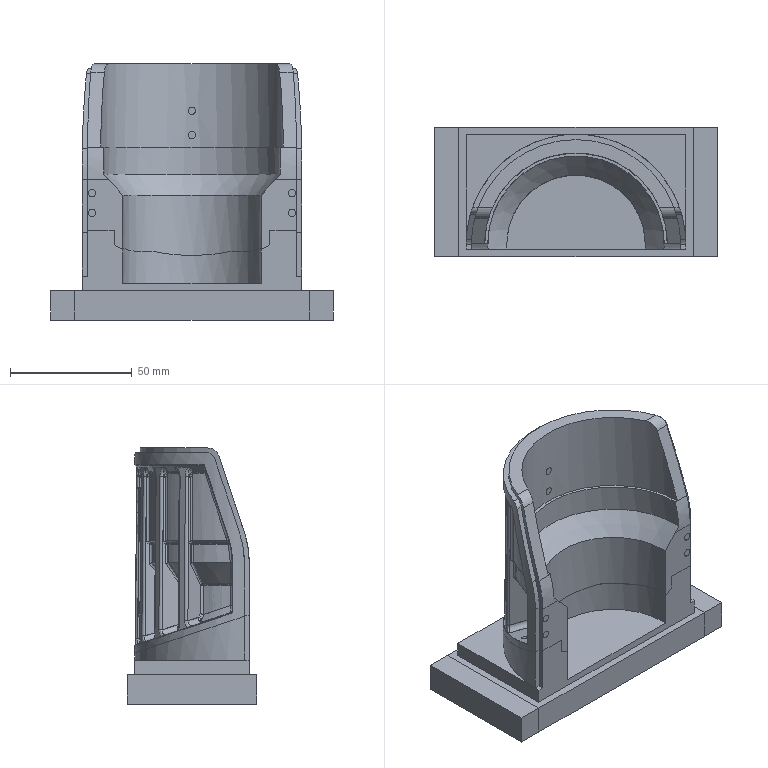NC program | NX | posted by the shop | part box 116 x 53 x 105 mm
Lines 39158 to 40130 of 44585:
T8 M6
;(T8:J-D2R1  D=2. R=1.)
;(XY=0.mm Z=0.mm)
G54 G90 D1
G0 A0.0 C=DC(0.0)
CYCLE832(0.04,_TOP_SURFACE_SMOOTH_ON+_ORI_SEMIFIN,1.)
G0 X32.535 Y1.7008 S9000 M3 M8
Z34.
Z-11.3
G1 Z-15.989 F3500.
G3 X32.535 Y.287 I.707 J-.707
G1 X32.687 Y.135 Z-16.078
X32.695 Y-.014 Z-16.083
X32.392 Y.289 Z-15.904
X32.248 Y.291 Z-15.82
X32.703 Y-.164 Z-16.088
X32.712 Y-.3131 Z-16.093
X32.105 Y.293 Z-15.737
X31.9625 Y.295 Z-15.657
X32.719 Y-.462 Z-16.097
X32.726 Y-.61 Z-16.102
X32.273 Y-.156 Z-15.834
X31.82 Y.296 Z-15.577
X31.678 Y.297 Z-15.5
X32.205 Y-.23 Z-15.794
X32.733 Y-.757 Z-16.106
X32.739 Y-.904 Z-16.109
X32.137 Y-.303 Z-15.755
X31.5361 Y.298 Z-15.423
X31.395 Y.299 Z-15.349
X32.0688 Y-.375 Z-15.716
X32.744 Y-1.05 Z-16.112
X32.748 Y-1.196 Z-16.1153
X32. Y-.448 Z-15.678
X31.253 Y.299 Z-15.275
X31.112 Y.3 Z-15.203
X31.532 Y-.12 Z-15.421
X31.932 Y-.52 Z-15.639
X32.3314 Y-.92 Z-15.868
X32.752 Y-1.34 Z-16.117
X32.755 Y-1.484 Z-16.119
X32.298 Y-1.028 Z-15.849
X31.862 Y-.592 Z-15.6002
X31.427 Y-.156 Z-15.365
X30.9706 Y.3 Z-15.1317
X30.829 Y.3 Z-15.061
X31.321 Y-.192 Z-15.31
X31.793 Y-.664 Z-15.562
X32.265 Y-1.135 Z-15.829
X32.757 Y-1.627 Z-16.1206
X32.758 Y-1.77 Z-16.122
X32.231 Y-1.242 Z-15.809
X31.723 Y-.735 Z-15.524
X31.216 Y-.227 Z-15.255
X30.688 Y.3 Z-14.992
X30.547 Y.3 Z-14.924
X31.11 Y-.263 Z-15.202
X31.653 Y-.806 Z-15.4864
X32.196 Y-1.349 Z-15.788
X32.759 Y-1.912 Z-16.122
X32.759 Y-2.053 Z-16.122
X32.161 Y-1.455 Z-15.768
X31.583 Y-.8764 Z-15.448
X31.004 Y-.298 Z-15.1485
X30.406 Y.3 Z-14.857
X30.265 Z-14.791
X30.899 Y-.333 Z-15.095
X31.512 Y-.947 Z-15.41
X32.125 Y-1.56 Z-15.748
X32.7585 Y-2.193 Z-16.122
X32.758 Y-2.3334 Z-16.121
X32.089 Y-1.665 Z-15.728
X31.441 Y-1.017 Z-15.373
X30.7926 Y-.368 Z-15.0429
X30.124 Y.3 Z-14.725
X29.983 Y.3 Z-14.661
X30.686 Y-.403 Z-14.991
X31.37 Y-1.086 Z-15.336
X32.053 Y-1.77 Z-15.7076
X32.7558 Y-2.473 Z-16.12
X32.754 Y-2.611 Z-16.119
X32.016 Y-1.874 Z-15.687
X31.298 Y-1.156 Z-15.298
X30.58 Y-.438 Z-14.94
X29.842 Y.3 Z-14.597
X29.701 Y.3 Z-14.535
X30.474 Y-.472 Z-14.888
X31.226 Y-1.225 Z-15.261
X31.978 Y-1.977 Z-15.6658
X32.75 Y-2.749 Z-16.117
X32.747 Y-2.886 Z-16.114
X32.334 Y-2.474 Z-15.869
X31.94 Y-2.08 Z-15.644
X31.154 Y-1.294 Z-15.224
X30.367 Y-.507 Z-14.838
X29.56 Y.3 Z-14.473
X29.419 Y.3 Z-14.411
X29.85 Y-.131 Z-14.601
X30.26 Y-.541 Z-14.788
X30.671 Y-.952 Z-14.984
X31.081 Y-1.362 Z-15.187
X31.492 Y-1.773 Z-15.3996
X31.902 Y-2.183 Z-15.622
X32.313 Y-2.594 Z-15.857
X32.743 Y-3.0237 Z-16.112
X32.739 Y-3.161 Z-16.11
X32.292 Y-2.714 Z-15.844
X31.864 Y-2.286 Z-15.601
X31.437 Y-1.8585 Z-15.371
X31.009 Y-1.431 Z-15.151
X30.581 Y-1.003 Z-14.9403
X30.154 Y-.576 Z-14.738
X29.726 Y-.148 Z-14.545
X29.278 Y.2999 Z-14.351
X29.1366 Y.301 Z-14.299
X29.157 Y.28 Z-14.305
X29.6015 Y-.164 Z-14.491
X30.046 Y-.609 Z-14.6895
X30.491 Y-1.054 Z-14.897
X30.936 Y-1.499 Z-15.114
X31.381 Y-1.944 Z-15.342
X31.826 Y-2.388 Z-15.58
X32.27 Y-2.833 Z-15.832
X32.735 Y-3.2974 Z-16.107
X32.729 Y-3.433 Z-16.104
X32.248 Y-2.9522 Z-15.819
X31.786 Y-2.49 Z-15.559
X31.325 Y-2.0285 Z-15.312
X30.863 Y-1.567 Z-15.077
X30.4009 Y-1.105 Z-14.854
X29.939 Y-.643 Z-14.641
X29.4772 Y-.181 Z-14.436
X29.246 Y.05 Z-14.337
X29.015 Y.281 Z-14.272
X28.995 Y.301 Z-14.269
X28.8553 Y.2998 Z-14.26
X28.875 Y.28 Z-14.26
X29.115 Y.041 Z-14.2928
X29.174 Y-.019 Z-14.31
X29.2342 Y-.0791 Z-14.332
X29.354 Y-.199 Z-14.383
X29.833 Y-.677 Z-14.593
X30.311 Y-1.156 Z-14.812
X30.79 Y-1.635 Z-15.042
X31.269 Y-2.114 Z-15.283
X31.747 Y-2.592 Z-15.538
X32.226 Y-3.071 Z-15.806
X32.724 Y-3.569 Z-16.1
X32.718 Y-3.704 Z-16.096
X32.203 Y-3.1891 Z-15.793
X31.708 Y-2.694 Z-15.516
X31.212 Y-2.198 Z-15.253
X30.717 Y-1.703 Z-15.006
X30.221 Y-1.207 Z-14.77
X29.7258 Y-.712 Z-14.545
X29.23 Y-.216 Z-14.331
X29.106 Y-.092 Z-14.291
X29.014 Y.001 Z-14.272
X28.983 Y.0315 Z-14.268
X28.735 Y.279 Z-14.268
X28.715 Y.299 Z-14.271
X28.623 Z-14.289
X28.574 Y.299 Z-14.303
X28.5939 Y.279 Z-14.297
X28.85 Y.023 Z-14.26
X28.914 Y-.041 Z-14.262
X28.978 Y-.105 Z-14.267
X29.106 Y-.233 Z-14.291
X29.362 Y-.489 Z-14.3865
X29.619 Y-.745 Z-14.498
X30.131 Y-1.258 Z-14.728
X30.643 Y-1.77 Z-14.97
X31.155 Y-2.282 Z-15.225
X31.668 Y-2.795 Z-15.494
X32.18 Y-3.307 Z-15.779
X32.7114 Y-3.838 Z-16.092
X32.705 Y-3.972 Z-16.088
X32.156 Y-3.424 Z-15.7661
X31.627 Y-2.895 Z-15.472
X31.098 Y-2.366 Z-15.196
X30.569 Y-1.8374 Z-14.935
X30.04 Y-1.3084 Z-14.687
X29.511 Y-.779 Z-14.451
X29.247 Y-.515 Z-14.338
X28.982 Y-.25 Z-14.2676
X28.85 Y-.118 Z-14.26
X28.751 Y-.019 Z-14.266
X28.718 Y.014 Z-14.271
X28.453 Y.279 Z-14.347
X28.434 Y.298 Z-14.356
X28.294 Y.297 Z-14.4368
X28.314 Y.277 Z-14.424
X28.45 Y.141 Z-14.349
X28.586 Y.005 Z-14.299
X28.655 Y-.0635 Z-14.282
X28.723 Y-.132 Z-14.27
X28.859 Y-.268 Z-14.26
X29.132 Y-.541 Z-14.297
X29.404 Y-.813 Z-14.405
X29.949 Y-1.358 Z-14.6457
X30.495 Y-1.904 Z-14.898
X31.04 Y-2.449 Z-15.166
X31.585 Y-2.994 Z-15.449
X32.13 Y-3.539 Z-15.751
X32.694 Y-4.103 Z-16.082
X32.684 Y-4.2337 Z-16.075
X32.104 Y-3.654 Z-15.737
X31.542 Y-3.092 Z-15.426
X30.981 Y-2.531 Z-15.137
X30.42 Y-1.97 Z-14.863
X29.858 Y-1.408 Z-14.604
X29.297 Y-.847 Z-14.359
X29.157 Y-.707 Z-14.305
X29.016 Y-.566 Z-14.272
X28.736 Y-.286 Z-14.268
X28.595 Y-.145 Z-14.296
X28.455 Y-.005 Z-14.347
X28.385 Y.0652 Z-14.3812
X28.315 Y.135 Z-14.423
X28.155 Y.295 Z-14.53
X28.016 Y.293 Z-14.622
X28.324 Y-.015 Z-14.417
X28.469 Y-.16 Z-14.3406
X28.613 Y-.304 Z-14.2916
X28.757 Y-.448 Z-14.266
X28.902 Y-.593 Z-14.261
X29.046 Y-.737 Z-14.277
X29.191 Y-.8815 Z-14.316
X29.768 Y-1.459 Z-14.564
X30.345 Y-2.036 Z-14.828
X30.923 Y-2.614 Z-15.107
X31.5 Y-3.191 Z-15.404
X32.077 Y-3.768 Z-15.722
X32.673 Y-4.364 Z-16.069
X32.662 Y-4.494 Z-16.062
X32.05 Y-3.882 Z-15.706
X31.457 Y-3.289 Z-15.381
X30.864 Y-2.696 Z-15.078
X30.27 Y-2.102 Z-14.793
X29.677 Y-1.509 Z-14.524
X29.381 Y-1.213 Z-14.394
X29.084 Y-.9159 Z-14.2853
X28.936 Y-.768 Z-14.263
X28.787 Y-.619 Z-14.263
X28.639 Y-.471 Z-14.285
X28.491 Y-.323 Z-14.332
X28.342 Y-.174 Z-14.406
X28.305 Y-.137 Z-14.429
X28.171 Y-.003 Z-14.519
X27.878 Y.29 Z-14.714
X27.74 Y.287 Z-14.807
X28.031 Y-.004 Z-14.613
X28.302 Y-.2749 Z-14.432
X28.3685 Y-.342 Z-14.39
X28.521 Y-.4938 Z-14.32
X28.673 Y-.646 Z-14.278
X28.825 Y-.798 Z-14.261
X28.978 Y-.951 Z-14.267
X29.13 Y-1.103 Z-14.297
X29.282 Y-1.2552 Z-14.352
X29.587 Y-1.56 Z-14.484
X30.196 Y-2.169 Z-14.758
X30.805 Y-2.778 Z-15.049
X31.414 Y-3.3871 Z-15.359
X32.023 Y-3.996 Z-15.691
X32.651 Y-4.6238 Z-16.055
X32.638 Y-4.753 Z-16.048
X31.996 Y-4.11 Z-15.6751
X31.372 Y-3.486 Z-15.337
X30.748 Y-2.862 Z-15.021
X30.124 Y-2.238 Z-14.725
X29.5 Y-1.614 Z-14.446
X29.188 Y-1.302 Z-14.315
X29.032 Y-1.1456 Z-14.275
X28.876 Y-.99 Z-14.26
X28.7195 Y-.834 Z-14.2704
X28.563 Y-.678 Z-14.306
X28.407 Y-.521 Z-14.3693
X28.31 Y-.424 Z-14.426
X28.305 Y-.4191 Z-14.429
X27.891 Y-.005 Z-14.706
X27.607 Y.279 Z-14.895
X27.607 Y.138 Z-14.895
X27.845 Y-.1004 Z-14.7362
X28.303 Y-.558 Z-14.431
X28.327 Y-.582 Z-14.415
X28.405 Y-.66 Z-14.371
X28.56 Y-.8155 Z-14.307
X28.716 Y-.971 Z-14.271
X28.872 Y-1.127 Z-14.26
X29.027 Y-1.283 Z-14.274
X29.183 Y-1.438 Z-14.313
X29.494 Y-1.75 Z-14.444
X30.117 Y-2.372 Z-14.722
X30.74 Y-2.995 Z-15.018
X31.362 Y-3.618 Z-15.332
X31.985 Y-4.24 Z-15.669
X32.626 Y-4.881 Z-16.04
X32.614 Y-5.01 Z-16.033
X31.974 Y-4.37 Z-15.6627
X31.353 Y-3.749 Z-15.327
X30.732 Y-3.128 Z-15.014
X30.111 Y-2.507 Z-14.719
X29.489 Y-1.885 Z-14.442
X29.179 Y-1.575 Z-14.312
X29.023 Y-1.419 Z-14.273
X28.868 Y-1.264 Z-14.26
X28.713 Y-1.1088 Z-14.2714
X28.557 Y-.953 Z-14.308
X28.4021 Y-.798 Z-14.372
X28.305 Y-.7011 Z-14.429
X27.8488 Y-.245 Z-14.734
X27.606 Y-.002 Z-14.896
X27.605 Y-.142 Z-14.8966
X27.847 Y-.384 Z-14.735
X28.303 Y-.84 Z-14.431
X28.399 Y-.937 Z-14.373
X28.554 Y-1.091 Z-14.3086
X28.709 Y-1.246 Z-14.272
X28.864 Y-1.401 Z-14.26
X29.019 Y-1.556 Z-14.273
X29.1742 Y-1.711 Z-14.31
X29.484 Y-2.0212 Z-14.44
X30.104 Y-2.641 Z-14.716
X30.724 Y-3.261 Z-15.01
X31.344 Y-3.881 Z-15.322
X31.963 Y-4.5005 Z-15.657
X32.602 Y-5.139 Z-16.0253
X32.589 Y-5.267 Z-16.017
X31.952 Y-4.63 Z-15.65
X31.334 Y-4.012 Z-15.317
X30.715 Y-3.394 Z-15.006
X30.097 Y-2.775 Z-14.713
X29.479 Y-2.157 Z-14.437
X29.17 Y-1.848 Z-14.3089
X29.015 Y-1.6931 Z-14.272
X28.86 Y-1.539 Z-14.26
X28.706 Y-1.384 Z-14.272
X28.551 Y-1.229 Z-14.31
X28.397 Y-1.075 Z-14.375
X28.305 Y-.983 Z-14.43
X27.846 Y-.524 Z-14.736
X27.604 Y-.282 Z-14.8972
X27.603 Y-.4221 Z-14.8978
X27.849 Y-.668 Z-14.734
X28.302 Y-1.121 Z-14.431
X28.394 Y-1.213 Z-14.376
X28.548 Y-1.367 Z-14.311
X28.702 Y-1.521 Z-14.273
X28.8564 Y-1.676 Z-14.26
X29.0106 Y-1.83 Z-14.271
X29.165 Y-1.984 Z-14.307
X29.473 Y-2.2923 Z-14.435
X30.09 Y-2.909 Z-14.709
X30.707 Y-3.526 Z-15.002
X31.3235 Y-4.143 Z-15.311
X31.94 Y-4.7594 Z-15.643
X32.575 Y-5.394 Z-16.009
X32.561 Y-5.522 Z-16.001
X31.928 Y-4.8883 Z-15.637
X31.313 Y-4.273 Z-15.306
X30.698 Y-3.658 Z-14.997
X30.083 Y-3.043 Z-14.706
X29.467 Y-2.428 Z-14.432
X29.16 Y-2.12 Z-14.3056
X29.0061 Y-1.966 Z-14.271
X28.8523 Y-1.812 Z-14.26
X28.699 Y-1.659 Z-14.274
X28.545 Y-1.505 Z-14.312
X28.391 Y-1.351 Z-14.378
X28.304 Y-1.265 Z-14.43
X27.848 Y-.808 Z-14.735
X27.602 Y-.562 Z-14.898
X27.601 Y-.702 Z-14.899
X27.846 Y-.947 Z-14.736
X28.302 Y-1.403 Z-14.432
X28.388 Y-1.489 Z-14.38
X28.541 Y-1.642 Z-14.313
X28.695 Y-1.796 Z-14.274
X28.848 Y-1.949 Z-14.26
X29.001 Y-2.1025 Z-14.27
X29.155 Y-2.256 Z-14.304
X29.461 Y-2.5626 Z-14.43
X30.075 Y-3.176 Z-14.703
X30.688 Y-3.79 Z-14.993
X31.302 Y-4.403 Z-15.3
X31.915 Y-5.016 Z-15.6294
X32.5468 Y-5.648 Z-15.992
X32.532 Y-5.774 Z-15.9837
X31.902 Y-5.145 Z-15.622
X31.291 Y-4.533 Z-15.294
X30.679 Y-3.921 Z-14.988
X30.067 Y-3.309 Z-14.699
X29.455 Y-2.698 Z-14.427
X29.15 Y-2.392 Z-14.302
X28.997 Y-2.239 Z-14.269
X28.844 Y-2.086 Z-14.26
X28.691 Y-1.9329 Z-14.275
X28.538 Y-1.78 Z-14.314
X28.385 Y-1.627 Z-14.381
X28.304 Y-1.546 Z-14.43
X27.85 Y-1.092 Z-14.733
X27.6003 Y-.842 Z-14.9
X27.5994 Y-.983 Z-14.9
X27.848 Y-1.231 Z-14.7344
X28.306 Y-1.689 Z-14.429
X28.382 Y-1.765 Z-14.383
X28.534 Y-1.918 Z-14.3153
X28.687 Y-2.07 Z-14.275
X28.839 Y-2.223 Z-14.259
X28.992 Y-2.375 Z-14.2674
X29.144 Y-2.528 Z-14.3
X29.449 Y-2.833 Z-14.424
X30.059 Y-3.443 Z-14.696
X30.669 Y-4.053 Z-14.984
X31.28 Y-4.663 Z-15.288
X31.89 Y-5.273 Z-15.615
X32.518 Y-5.901 Z-15.975
X32.503 Y-6.027 Z-15.966
X31.877 Y-5.401 Z-15.608
X31.268 Y-4.793 Z-15.282
X30.66 Y-4.184 Z-14.979
X30.052 Y-3.576 Z-14.692
X29.443 Y-2.968 Z-14.422
X29.1392 Y-2.6634 Z-14.298
X28.987 Y-2.511 Z-14.266
X28.835 Y-2.359 Z-14.259
X28.683 Y-2.207 Z-14.275
X28.531 Y-2.055 Z-14.316
X28.379 Y-1.903 Z-14.384
X28.303 Y-1.827 Z-14.431
X27.8465 Y-1.3707 Z-14.735
X27.599 Y-1.1227 Z-14.901
X27.598 Y-1.263 Z-14.901
X27.845 Y-1.5101 Z-14.7365
X28.304 Y-1.97 Z-14.4298
X28.376 Y-2.041 Z-14.386
X28.527 Y-2.192 Z-14.316
X28.679 Y-2.344 Z-14.275
X28.83 Y-2.496 Z-14.258
X28.982 Y-2.647 Z-14.265
X29.134 Y-2.799 Z-14.296
X29.437 Y-3.102 Z-14.419
X30.043 Y-3.708 Z-14.688
X30.65 Y-4.315 Z-14.974
X31.256 Y-4.921 Z-15.276
X31.862 Y-5.5276 Z-15.6
X32.487 Y-6.152 Z-15.956
X32.4701 Y-6.276 Z-15.946
X31.848 Y-5.654 Z-15.592
X31.243 Y-5.05 Z-15.2695
X30.6389 Y-4.445 Z-14.968
X30.034 Y-3.841 Z-14.684
X29.43 Y-3.236 Z-14.416
X29.128 Y-2.934 Z-14.2934
X28.977 Y-2.783 Z-14.263
X28.826 Y-2.632 Z-14.257
X28.6744 Y-2.481 Z-14.275
X28.523 Y-2.33 Z-14.316
X28.372 Y-2.1784 Z-14.386
X28.193 Y-1.999 Z-14.504
X27.848 Y-1.654 Z-14.734
X27.597 Y-1.403 Z-14.902
X27.596 Y-1.543 Z-14.902
X27.846 Y-1.794 Z-14.736
X28.049 Y-1.996 Z-14.601
X28.218 Y-2.165 Z-14.485
X28.369 Y-2.3159 Z-14.387
X28.519 Y-2.466 Z-14.316
X28.67 Y-2.617 Z-14.274
X28.82 Y-2.768 Z-14.255
X28.971 Y-2.918 Z-14.261
X29.122 Y-3.069 Z-14.291
X29.4228 Y-3.37 Z-14.413
X30.025 Y-3.972 Z-14.68
X30.628 Y-4.575 Z-14.963
X31.23 Y-5.177 Z-15.263
X31.832 Y-5.78 Z-15.584
X32.452 Y-6.399 Z-15.936
X32.434 Y-6.522 Z-15.925
X31.816 Y-5.904 Z-15.575
X31.216 Y-5.304 Z-15.2553
X30.616 Y-4.704 Z-14.9569
X30.015 Y-4.104 Z-14.6757
X29.415 Y-3.504 Z-14.41
X29.115 Y-3.203 Z-14.288
X28.965 Y-3.053 Z-14.258
X28.815 Y-2.9034 Z-14.2533
X28.6651 Y-2.753 Z-14.272
X28.515 Y-2.603 Z-14.317
X28.365 Y-2.453 Z-14.387
X28.215 Y-2.303 Z-14.485
X27.595 Y-1.683 Z-14.903
X27.594 Y-1.823 Z-14.904
X28.212 Y-2.441 Z-14.485
X28.361 Y-2.591 Z-14.388
X28.511 Y-2.74 Z-14.315
X28.66 Y-2.89 Z-14.27
X28.81 Y-3.039 Z-14.251
X28.959 Y-3.189 Z-14.256
X29.109 Y-3.338 Z-14.286
X29.408 Y-3.637 Z-14.406
X30.006 Y-4.235 Z-14.671
X30.604 Y-4.833 Z-14.951
X31.202 Y-5.431 Z-15.248
X31.7997 Y-6.029 Z-15.566
X32.415 Y-6.645 Z-15.914
X32.397 Y-6.767 Z-15.903
X31.783 Y-6.1537 Z-15.557
X31.188 Y-5.558 Z-15.2409
X30.592 Y-4.962 Z-14.945
X29.9961 Y-4.366 Z-14.667
X29.4 Y-3.771 Z-14.403
X29.102 Y-3.473 Z-14.283
X28.9535 Y-3.324 Z-14.254
X28.805 Y-3.175 Z-14.249
X28.656 Y-3.0259 Z-14.268
X28.507 Y-2.877 Z-14.313
X28.358 Y-2.728 Z-14.385
X27.593 Y-1.963 Z-14.904
X27.592 Y-2.103 Z-14.904
X28.354 Y-2.8652 Z-14.383
X28.502 Y-3.014 Z-14.31
X28.651 Y-3.162 Z-14.266
X28.799 Y-3.31 Z-14.247
X28.947 Y-3.459 Z-14.251
X29.096 Y-3.607 Z-14.28
X29.393 Y-3.904 Z-14.4
X29.986 Y-4.498 Z-14.663
X30.58 Y-5.091 Z-14.939
X31.173 Y-5.685 Z-15.234
X31.767 Y-6.278 Z-15.548
X32.378 Y-6.889 Z-15.892
X32.359 Y-7.011 Z-15.881
X31.75 Y-6.402 Z-15.538
X31.158 Y-5.811 Z-15.226
X30.567 Y-5.219 Z-14.933
X29.976 Y-4.628 Z-14.6577
X29.384 Y-4.0366 Z-14.396
X29.0886 Y-3.741 Z-14.277
X28.941 Y-3.593 Z-14.248
X28.793 Y-3.445 Z-14.244
X28.645 Y-3.297 Z-14.264
X28.497 Y-3.15 Z-14.309
X28.349 Y-3.002 Z-14.381
X27.59 Y-2.243 Z-14.904
X27.5886 Y-2.382 Z-14.904
X28.345 Y-3.138 Z-14.379
X28.492 Y-3.285 Z-14.307
X28.639 Y-3.433 Z-14.261
X28.787 Y-3.58 Z-14.241
X28.934 Y-3.727 Z-14.244
X29.081 Y-3.874 Z-14.273
X29.376 Y-4.169 Z-14.393
X29.965 Y-4.758 Z-14.653
X30.554 Y-5.347 Z-14.927
X31.143 Y-5.9365 Z-15.2185
X31.732 Y-6.526 Z-15.529
X32.339 Y-7.132 Z-15.869
X32.318 Y-7.253 Z-15.857
X31.714 Y-6.649 Z-15.519
X31.1272 Y-6.062 Z-15.21
X30.54 Y-5.475 Z-14.92
X29.953 Y-4.888 Z-14.648
X29.366 Y-4.301 Z-14.389
X29.073 Y-4.007 Z-14.269
X28.926 Y-3.86 Z-14.241
X28.779 Y-3.7137 Z-14.237
X28.633 Y-3.567 Z-14.258
X28.486 Y-3.42 Z-14.303
X28.339 Y-3.273 Z-14.377
X28.192 Y-3.127 Z-14.478
X27.586 Y-2.52 Z-14.903
X27.583 Y-2.658 Z-14.902
X28.187 Y-3.263 Z-14.475
X28.333 Y-3.4087 Z-14.374
X28.48 Y-3.555 Z-14.3
X28.626 Y-3.701 Z-14.254
X28.772 Y-3.847 Z-14.2337
X28.918 Y-3.993 Z-14.237
X29.064 Y-4.14 Z-14.266
X29.357 Y-4.432 Z-14.384
X29.941 Y-5.017 Z-14.642
X30.526 Y-5.601 Z-14.913
X31.111 Y-6.186 Z-15.202
X31.6956 Y-6.771 Z-15.509
X32.298 Y-7.373 Z-15.845
X32.276 Y-7.4926 Z-15.832
X31.677 Y-6.893 Z-15.498
X31.094 Y-6.31 Z-15.194
X30.511 Y-5.728 Z-14.906
X29.929 Y-5.145 Z-14.637
X29.346 Y-4.563 Z-14.38
X29.055 Y-4.271 Z-14.261
X28.909 Y-4.1257 Z-14.233
X28.764 Y-3.98 Z-14.2298
X28.618 Y-3.834 Z-14.25
X28.472 Y-3.689 Z-14.296
X28.327 Y-3.543 Z-14.3702
X27.579 Y-2.795 Z-14.9
X27.575 Y-2.933 Z-14.899
X28.32 Y-3.677 Z-14.366
X28.465 Y-3.822 Z-14.292
X28.61 Y-3.967 Z-14.246
X28.755 Y-4.112 Z-14.226
X28.9001 Y-4.2575 Z-14.229
X29.045 Y-4.403 Z-14.257
X29.335 Y-4.693 Z-14.375
X29.9156 Y-5.273 Z-14.631
X30.496 Y-5.853 Z-14.899
X31.076 Y-6.434 Z-15.185
X31.656 Y-7.014 Z-15.487
X32.254 Y-7.611 Z-15.819
X32.232 Y-7.73 Z-15.806
X31.636 Y-7.135 Z-15.476
X31.058 Y-6.557 Z-15.176
X30.48 Y-5.978 Z-14.891
X29.902 Y-5.4 Z-14.624
X29.324 Y-4.822 Z-14.37
X29.035 Y-4.5331 Z-14.252
X28.89 Y-4.389 Z-14.224
X28.746 Y-4.244 Z-14.221
X28.601 Y-4.0995 Z-14.242
X28.457 Y-3.955 Z-14.288
X28.312 Y-3.81 Z-14.362
X28.167 Y-3.6659 Z-14.465
X27.57 Y-3.068 Z-14.896
X27.565 Y-3.2044 Z-14.893
X28.16 Y-3.8 Z-14.46
X28.304 Y-3.944 Z-14.358
X28.448 Y-4.088 Z-14.284
X28.592 Y-4.232 Z-14.238
X28.736 Y-4.376 Z-14.216
X28.88 Y-4.52 Z-14.22
X29.024 Y-4.664 Z-14.248
X29.312 Y-4.952 Z-14.365
X29.888 Y-5.528 Z-14.618
X30.464 Y-6.104 Z-14.884
X31.04 Y-6.68 Z-15.166
X31.616 Y-7.255 Z-15.465
X32.209 Y-7.8486 Z-15.794
X32.187 Y-7.967 Z-15.781
X31.596 Y-7.376 Z-15.4545
X31.022 Y-6.802 Z-15.157
X30.448 Y-6.228 Z-14.876
X29.874 Y-5.654 Z-14.612
X29.3 Y-5.08 Z-14.36
X29.013 Y-4.7932 Z-14.243
X28.869 Y-4.6497 Z-14.215
X28.726 Y-4.5062 Z-14.212
X28.582 Y-4.3627 Z-14.233
X28.439 Y-4.219 Z-14.279
X28.295 Y-4.076 Z-14.3535
X28.152 Y-3.932 Z-14.456
X27.559 Y-3.3391 Z-14.891
X27.552 Y-3.474 Z-14.888
X28.143 Y-4.065 Z-14.452
X28.286 Y-4.208 Z-14.349
X28.429 Y-4.351 Z-14.274
X28.572 Y-4.494 Z-14.228
X28.715 Y-4.637 Z-14.206
X28.858 Y-4.7797 Z-14.209
X29.001 Y-4.923 Z-14.238
X29.287 Y-5.209 Z-14.355
X29.859 Y-5.781 Z-14.605
X30.431 Y-6.353 Z-14.868
X31.003 Y-6.924 Z-15.148
X31.575 Y-7.496 Z-15.443
X32.164 Y-8.085 Z-15.768
X32.141 Y-8.203 Z-15.754
X31.554 Y-7.616 Z-15.432
X30.984 Y-7.046 Z-15.138
X30.414 Y-6.476 Z-14.8602
X29.843 Y-5.906 Z-14.598
X29.273 Y-5.336 Z-14.349
X28.988 Y-5.051 Z-14.2321
X28.846 Y-4.9084 Z-14.204
X28.703 Y-4.7659 Z-14.201
X28.561 Y-4.623 Z-14.222
X28.418 Y-4.481 Z-14.269
X28.2759 Y-4.338 Z-14.344
X27.544 Y-3.607 Z-14.884
X27.536 Y-3.7399 Z-14.881
X28.123 Y-4.3269 Z-14.442
X28.265 Y-4.469 Z-14.339
X28.407 Y-4.611 Z-14.263
X28.549 Y-4.753 Z-14.217
X28.692 Y-4.895 Z-14.196
X28.834 Y-5.037 Z-14.199
X28.976 Y-5.179 Z-14.226
X29.2596 Y-5.463 Z-14.343
X29.8277 Y-6.031 Z-14.591
X30.3958 Y-6.599 Z-14.8519
X30.9639 Y-7.167 Z-15.128
X31.532 Y-7.735 Z-15.42
X32.117 Y-8.32 Z-15.741
X32.092 Y-8.437 Z-15.726
X31.509 Y-7.854 Z-15.408
X30.943 Y-7.287 Z-15.117
X30.377 Y-6.7212 Z-14.843
X29.81 Y-6.155 Z-14.583
X29.244 Y-5.589 Z-14.336
X28.961 Y-5.306 Z-14.22
X28.82 Y-5.164 Z-14.193
X28.678 Y-5.023 Z-14.19
X28.5365 Y-4.881 Z-14.212
X28.395 Y-4.739 Z-14.258
X28.2534 Y-4.5979 Z-14.334
X28.112 Y-4.456 Z-14.438
X27.527 Y-3.871 Z-14.878
X27.517 Y-4.003 Z-14.874
X28.1 Y-4.586 Z-14.432
X28.241 Y-4.727 Z-14.328
X28.382 Y-4.868 Z-14.253
X28.523 Y-5.009 Z-14.206
X28.664 Y-5.15 Z-14.184
X28.8055 Y-5.291 Z-14.1865
X28.947 Y-5.432 Z-14.2141
X29.229 Y-5.714 Z-14.329
X29.793 Y-6.279 Z-14.5752
X30.357 Y-6.843 Z-14.834
X30.922 Y-7.407 Z-15.107
X31.4862 Y-7.972 Z-15.396
X32.067 Y-8.553 Z-15.712
X32.042 Y-8.668 Z-15.698
X31.4625 Y-8.089 Z-15.384
X30.9 Y-7.527 Z-15.0961
X30.337 Y-6.964 Z-14.825
X29.775 Y-6.401 Z-14.567
X29.212 Y-5.839 Z-14.323
X28.931 Y-5.558 Z-14.208
X28.791 Y-5.417 Z-14.18
X28.65 Y-5.276 Z-14.178
X28.5093 Y-5.136 Z-14.2
X28.369 Y-4.995 Z-14.247
X28.228 Y-4.855 Z-14.323
X28.087 Y-4.714 Z-14.428
X27.506 Y-4.133 Z-14.87
X27.495 Y-4.263 Z-14.866
X28.074 Y-4.842 Z-14.423
X28.215 Y-4.982 Z-14.318
X28.355 Y-5.122 Z-14.241
X28.495 Y-5.2625 Z-14.194
X28.635 Y-5.403 Z-14.171
X28.775 Y-5.543 Z-14.174
X28.915 Y-5.683 Z-14.201
X29.1958 Y-5.963 Z-14.316
X29.756 Y-6.524 Z-14.559
X30.317 Y-7.0847 Z-14.815
X30.878 Y-7.645 Z-15.085
X31.4385 Y-8.206 Z-15.371
X32.016 Y-8.783 Z-15.6832
X31.99 Y-8.899 Z-15.669
X31.414 Y-8.323 Z-15.359
X30.856 Y-7.764 Z-15.075
X30.297 Y-7.205 Z-14.805
X29.7377 Y-6.646 Z-14.551
X29.179 Y-6.087 Z-14.308
X28.899 Y-5.8079 Z-14.194
X28.76 Y-5.668 Z-14.167
X28.62 Y-5.528 Z-14.165
X28.48 Y-5.389 Z-14.187
X28.34 Y-5.249 Z-14.235
X28.2007 Y-5.109 Z-14.312
X28.061 Y-4.97 Z-14.417
X27.484 Y-4.392 Z-14.862
X27.4715 Y-4.521 Z-14.858
X28.047 Y-5.097 Z-14.411
X28.186 Y-5.236 Z-14.305
X28.326 Y-5.375 Z-14.228
X28.465 Y-5.515 Z-14.181
X28.604 Y-5.654 Z-14.158
X28.744 Y-5.793 Z-14.16
X28.883 Y-5.932 Z-14.187
X29.161 Y-6.211 Z-14.301
X29.719 Y-6.768 Z-14.542
X30.276 Y-7.325 Z-14.796
X30.8331 Y-7.883 Z-15.064
X31.39 Y-8.44 Z-15.346
X31.964 Y-9.014 Z-15.654
X31.938 Y-9.129 Z-15.64
X31.366 Y-8.557 Z-15.333
X30.811 Y-8.001 Z-15.053
X30.255 Y-7.446 Z-14.786
X29.699 Y-6.89 Z-14.534
X29.144 Y-6.335 Z-14.2934
X28.866 Y-6.057 Z-14.18
X28.727 Y-5.918 Z-14.153
X28.588 Y-5.779 Z-14.152
X28.449 Y-5.64 Z-14.1742
X28.3106 Y-5.5012 Z-14.222
X28.172 Y-5.362 Z-14.298
X28.033 Y-5.223 Z-14.404
X27.459 Y-4.65 Z-14.852
X27.446 Y-4.777 Z-14.848
X28.0179 Y-5.35 Z-14.398
X28.156 Y-5.488 Z-14.292
X28.295 Y-5.626 Z-14.215
X28.433 Y-5.765 Z-14.167
X28.572 Y-5.903 Z-14.144
X28.71 Y-6.0419 Z-14.1458
X28.849 Y-6.18 Z-14.173
X29.126 Y-6.457 Z-14.285
X29.68 Y-7.011 Z-14.525
X30.234 Y-7.565 Z-14.776
X30.787 Y-8.119 Z-15.041
X31.341 Y-8.673 Z-15.32
X31.912 Y-9.244 Z-15.625
X31.885 Y-9.358 Z-15.611
X31.3165 Y-8.789 Z-15.307
X30.764 Y-8.237 Z-15.03
X30.212 Y-7.685 Z-14.766
X29.66 Y-7.1323 Z-14.516
X29.107 Y-6.58 Z-14.277
X28.831 Y-6.304 Z-14.165
X28.693 Y-6.166 Z-14.138
X28.555 Y-6.028 Z-14.137
X28.417 Y-5.89 Z-14.16
X28.279 Y-5.752 Z-14.208
X28.141 Y-5.614 Z-14.285
X28.003 Y-5.475 Z-14.391
X27.432 Y-4.905 Z-14.842
X27.418 Y-5.032 Z-14.837
X27.9869 Y-5.601 Z-14.385
X28.125 Y-5.7382 Z-14.279
X28.262 Y-5.876 Z-14.201
X28.4 Y-6.014 Z-14.152
X28.538 Y-6.151 Z-14.1291
X28.675 Y-6.289 Z-14.131
X28.813 Y-6.426 Z-14.158
X29.088 Y-6.702 Z-14.269
X29.6388 Y-7.252 Z-14.507
X30.189 Y-7.803 Z-14.755
X30.74 Y-8.354 Z-15.018
X31.2907 Y-8.904 Z-15.294
X31.858 Y-9.471 Z-15.595
X31.829 Y-9.583 Z-15.579
X31.264 Y-9.018 Z-15.28
X30.715 Y-8.469 Z-15.005
X30.166 Y-7.921 Z-14.744
X29.617 Y-7.372 Z-14.498
X29.068 Y-6.823 Z-14.261
X28.794 Y-6.549 Z-14.15
X28.657 Y-6.411 Z-14.123
X28.52 Y-6.274 Z-14.122
X28.382 Y-6.137 Z-14.144
X28.245 Y-6. Z-14.193
X28.108 Y-5.863 Z-14.271
X27.971 Y-5.725 Z-14.378
X27.404 Y-5.159 Z-14.831
X27.389 Y-5.285 Z-14.8241
X27.954 Y-5.8496 Z-14.37
X28.091 Y-5.986 Z-14.263
X28.227 Y-6.123 Z-14.185
X28.364 Y-6.26 Z-14.137
X28.501 Y-6.397 Z-14.114
X28.638 Y-6.533 Z-14.116
X28.775 Y-6.67 Z-14.142
X29.048 Y-6.944 Z-14.252
X29.595 Y-7.491 Z-14.488
X30.142 Y-8.038 Z-14.7334
X30.689 Y-8.585 Z-14.993
X31.2363 Y-9.132 Z-15.266
X31.8 Y-9.695 Z-15.563
X31.7708 Y-9.807 Z-15.547
X31.209 Y-9.246 Z-15.252
X30.664 Y-8.7004 Z-14.98
X30.118 Y-8.155 Z-14.722
X29.573 Y-7.61 Z-14.479
X29.028 Y-7.064 Z-14.243
X28.755 Y-6.792 Z-14.134
X28.619 Y-6.655 Z-14.107
X28.482 Y-6.519 Z-14.1064
X28.346 Y-6.383 Z-14.129
X28.21 Y-6.246 Z-14.177
X28.073 Y-6.11 Z-14.254
X27.937 Y-5.9737 Z-14.362
X27.3737 Y-5.41 Z-14.818
X27.359 Y-5.536 Z-14.811
X27.92 Y-6.098 Z-14.354
X28.056 Y-6.234 Z-14.246
X28.192 Y-6.37 Z-14.17
X28.328 Y-6.506 Z-14.121
X28.464 Y-6.641 Z-14.098
X28.6 Y-6.777 Z-14.099
X28.736 Y-6.913 Z-14.126
X29.007 Y-7.185 Z-14.235
X29.551 Y-7.729 Z-14.469
X30.095 Y-8.272 Z-14.712
X30.638 Y-8.816 Z-14.968
X31.182 Y-9.359 Z-15.238
X31.742 Y-9.92 Z-15.532
X31.713 Y-10.031 Z-15.516
X31.154 Y-9.473 Z-15.224
X30.612 Y-8.9308 Z-14.955
X30.07 Y-8.389 Z-14.701
X29.528 Y-7.8467 Z-14.459
X28.986 Y-7.305 Z-14.226
X28.715 Y-7.034 Z-14.117
X28.5794 Y-6.898 Z-14.091
X28.444 Y-6.763 Z-14.089
X28.308 Y-6.6271 Z-14.113
X28.173 Y-6.492 Z-14.162
X28.037 Y-6.356 Z-14.239
X27.902 Y-6.221 Z-14.346
X27.342 Y-5.661 Z-14.805
X27.3246 Y-5.784 Z-14.798
X27.883 Y-6.342 Z-14.339
X28.018 Y-6.478 Z-14.232
X28.153 Y-6.613 Z-14.153
X28.288 Y-6.748 Z-14.104
X28.423 Y-6.883 Z-14.081
X28.558 Y-7.018 Z-14.082
X28.693 Y-7.1532 Z-14.109
X28.964 Y-7.423 Z-14.2163
X29.504 Y-7.964 Z-14.4486
X30.045 Y-8.505 Z-14.689
X30.585 Y-9.045 Z-14.942
X31.126 Y-9.586 Z-15.2097
X31.6828 Y-10.143 Z-15.5
X31.6531 Y-10.254 Z-15.4837
X31.098 Y-9.698 Z-15.195
X30.558 Y-9.159 Z-14.929
X30.019 Y-8.62 Z-14.678
X29.48 Y-8.081 Z-14.438
X28.941 Y-7.541 Z-14.207
X28.671 Y-7.272 Z-14.1
X28.536 Y-7.137 Z-14.073
X28.401 Y-7.002 Z-14.072
X28.267 Y-6.867 Z-14.096
X28.132 Y-6.7326 Z-14.145
X27.997 Y-6.5978 Z-14.223
X27.862 Y-6.463 Z-14.332
X27.306 Y-5.906 Z-14.792
X27.286 Y-6.028 Z-14.785
X27.842 Y-6.5836 Z-14.324
X27.976 Y-6.718 Z-14.2149
X28.111 Y-6.853 Z-14.1366
X28.245 Y-6.987 Z-14.0875
X28.38 Y-7.121 Z-14.064
X28.5142 Y-7.256 Z-14.064
X28.649 Y-7.39 Z-14.0904
X28.918 Y-7.659 Z-14.197
X29.4555 Y-8.197 Z-14.427
X29.993 Y-8.735 Z-14.666
X30.531 Y-9.273 Z-14.916
X31.069 Y-9.811 Z-15.1808
X31.623 Y-10.365 Z-15.468
X31.594 Y-10.476 Z-15.452
X31.041 Y-9.924 Z-15.166
X30.504 Y-9.387 Z-14.903
X29.968 Y-8.85 Z-14.654
X29.431 Y-8.314 Z-14.417
X28.895 Y-7.777 Z-14.187
X28.626 Y-7.509 Z-14.081
X28.492 Y-7.375 Z-14.055
X28.358 Y-7.241 Z-14.055
X28.224 Y-7.107 Z-14.079
X28.09 Y-6.972 Z-14.128
X27.956 Y-6.838 Z-14.206
X27.821 Y-6.704 Z-14.315
X27.267 Y-6.15 Z-14.778
X27.248 Y-6.272 Z-14.771
X27.801 Y-6.825 Z-14.307
X27.935 Y-6.959 Z-14.198
X28.068 Y-7.092 Z-14.1201
X28.202 Y-7.226 Z-14.07
X28.336 Y-7.36 Z-14.046
X28.47 Y-7.494 Z-14.046
X28.604 Y-7.627 Z-14.072
X28.871 Y-7.895 Z-14.178
X29.406 Y-8.43 Z-14.406
X29.941 Y-8.965 Z-14.6423